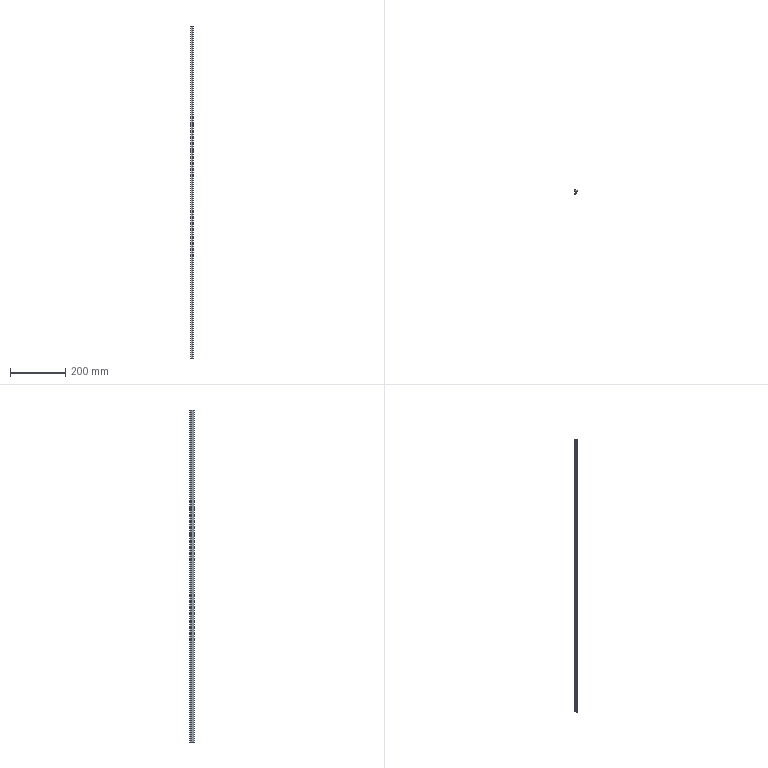Part | SolidWorks | features BaseBody 1, MoveFace 1 | 1 solid | 20 faces | box 10.8 x 17.5 x 1197 mm | volume 94324 mm3 | cylinder 11 | plane 9 | commonest cylinder face diameters 1.6 x2 14 x2 0.4 x1 0.6 x1 0.8 x1 2.6 x1
STEP:
#1=CARTESIAN_POINT('',(-3.236,-11.055,1097.));
#2=VERTEX_POINT('',#1);
#3=CARTESIAN_POINT('',(-4.3,-10.3,1097.));
#4=VERTEX_POINT('',#3);
#5=CARTESIAN_POINT('',(-3.5,-10.3,1097.));
#6=DIRECTION('',(0.,0.,-1.));
#7=DIRECTION('',(1.,0.,0.));
#8=AXIS2_PLACEMENT_3D('',#5,#6,#7);
#9=CIRCLE('',#8,0.8);
#10=EDGE_CURVE('',#2,#4,#9,.T.);
#11=ORIENTED_EDGE('',*,*,#10,.T.);
#12=CARTESIAN_POINT('',(-4.3,-10.3,-100.));
#13=VERTEX_POINT('',#12);
#14=CARTESIAN_POINT('',(-4.3,-10.3,-100.));
#15=DIRECTION('',(0.,0.,-1.));
#16=VECTOR('',#15,1000.);
#17=LINE('',#14,#16);
#18=EDGE_CURVE('',#4,#13,#17,.T.);
#19=ORIENTED_EDGE('',*,*,#18,.T.);
#20=CARTESIAN_POINT('',(-3.236,-11.055,-100.));
#21=VERTEX_POINT('',#20);
#22=CARTESIAN_POINT('',(-3.5,-10.3,-100.));
#23=DIRECTION('',(0.,0.,1.));
#24=DIRECTION('',(-1.,0.,0.));
#25=AXIS2_PLACEMENT_3D('',#22,#23,#24);
#26=CIRCLE('',#25,0.8);
#27=EDGE_CURVE('',#13,#21,#26,.T.);
#28=ORIENTED_EDGE('',*,*,#27,.T.);
#29=CARTESIAN_POINT('',(-3.236,-11.055,-100.));
#30=DIRECTION('',(0.,0.,-1.));
#31=VECTOR('',#30,1000.);
#32=LINE('',#29,#31);
#33=EDGE_CURVE('',#2,#21,#32,.T.);
#34=ORIENTED_EDGE('',*,*,#33,.F.);
#35=EDGE_LOOP('',(#11,#19,#28,#34));
#36=FACE_OUTER_BOUND('',#35,.T.);
#37=CARTESIAN_POINT('',(-3.5,-10.3,-100.));
#38=DIRECTION('',(0.,0.,-1.));
#39=DIRECTION('',(-1.,0.,0.));
#40=AXIS2_PLACEMENT_3D('',#37,#38,#39);
#41=CYLINDRICAL_SURFACE('',#40,0.8);
#42=ADVANCED_FACE('',(#36),#41,.T.);
#43=CARTESIAN_POINT('',(1.184,-6.397,-100.));
#44=VERTEX_POINT('',#43);
#45=CARTESIAN_POINT('',(-5.702,-4.29,-100.));
#46=DIRECTION('',(0.,0.,1.));
#47=DIRECTION('',(-1.,0.,0.));
#48=AXIS2_PLACEMENT_3D('',#45,#46,#47);
#49=CIRCLE('',#48,7.201);
#50=EDGE_CURVE('',#21,#44,#49,.T.);
#51=ORIENTED_EDGE('',*,*,#50,.T.);
#52=CARTESIAN_POINT('',(1.184,-6.397,1097.));
#53=VERTEX_POINT('',#52);
#54=CARTESIAN_POINT('',(1.184,-6.397,-100.));
#55=DIRECTION('',(0.,0.,1.));
#56=VECTOR('',#55,1000.);
#57=LINE('',#54,#56);
#58=EDGE_CURVE('',#44,#53,#57,.T.);
#59=ORIENTED_EDGE('',*,*,#58,.T.);
#60=CARTESIAN_POINT('',(-5.702,-4.29,1097.));
#61=DIRECTION('',(0.,0.,-1.));
#62=DIRECTION('',(1.,0.,0.));
#63=AXIS2_PLACEMENT_3D('',#60,#61,#62);
#64=CIRCLE('',#63,7.201);
#65=EDGE_CURVE('',#53,#2,#64,.T.);
#66=ORIENTED_EDGE('',*,*,#65,.T.);
#67=ORIENTED_EDGE('',*,*,#33,.T.);
#68=EDGE_LOOP('',(#51,#59,#66,#67));
#69=FACE_OUTER_BOUND('',#68,.T.);
#70=CARTESIAN_POINT('',(-5.702,-4.29,-100.));
#71=DIRECTION('',(0.,0.,-1.));
#72=DIRECTION('',(-1.,0.,0.));
#73=AXIS2_PLACEMENT_3D('',#70,#71,#72);
#74=CYLINDRICAL_SURFACE('',#73,7.201);
#75=ADVANCED_FACE('',(#69),#74,.T.);
#76=CARTESIAN_POINT('',(0.9,-6.,-100.));
#77=VERTEX_POINT('',#76);
#78=CARTESIAN_POINT('',(0.9,-6.3,-100.));
#79=DIRECTION('',(0.,0.,1.));
#80=DIRECTION('',(-1.,0.,0.));
#81=AXIS2_PLACEMENT_3D('',#78,#79,#80);
#82=CIRCLE('',#81,0.3);
#83=EDGE_CURVE('',#44,#77,#82,.T.);
#84=ORIENTED_EDGE('',*,*,#83,.T.);
#85=CARTESIAN_POINT('',(0.9,-6.,1097.));
#86=VERTEX_POINT('',#85);
#87=CARTESIAN_POINT('',(0.9,-6.,-100.));
#88=DIRECTION('',(0.,0.,1.));
#89=VECTOR('',#88,1000.);
#90=LINE('',#87,#89);
#91=EDGE_CURVE('',#77,#86,#90,.T.);
#92=ORIENTED_EDGE('',*,*,#91,.T.);
#93=CARTESIAN_POINT('',(0.9,-6.3,1097.));
#94=DIRECTION('',(0.,0.,-1.));
#95=DIRECTION('',(1.,0.,0.));
#96=AXIS2_PLACEMENT_3D('',#93,#94,#95);
#97=CIRCLE('',#96,0.3);
#98=EDGE_CURVE('',#86,#53,#97,.T.);
#99=ORIENTED_EDGE('',*,*,#98,.T.);
#100=ORIENTED_EDGE('',*,*,#58,.F.);
#101=EDGE_LOOP('',(#84,#92,#99,#100));
#102=FACE_OUTER_BOUND('',#101,.T.);
#103=CARTESIAN_POINT('',(0.9,-6.3,-100.));
#104=DIRECTION('',(0.,0.,-1.));
#105=DIRECTION('',(-1.,0.,0.));
#106=AXIS2_PLACEMENT_3D('',#103,#104,#105);
#107=CYLINDRICAL_SURFACE('',#106,0.3);
#108=ADVANCED_FACE('',(#102),#107,.T.);
#109=CARTESIAN_POINT('',(-2.5,-0.5,-100.));
#110=VERTEX_POINT('',#109);
#111=CARTESIAN_POINT('',(-2.5,-6.153,-100.));
#112=VERTEX_POINT('',#111);
#113=CARTESIAN_POINT('',(-2.5,-6.397,-100.));
#114=DIRECTION('',(0.,-1.,0.));
#115=VECTOR('',#114,1000.);
#116=LINE('',#113,#115);
#117=EDGE_CURVE('',#110,#112,#116,.T.);
#118=ORIENTED_EDGE('',*,*,#117,.F.);
#119=CARTESIAN_POINT('',(-4.2,1.695,-100.));
#120=VERTEX_POINT('',#119);
#121=CARTESIAN_POINT('',(-1.701,1.875,-100.));
#122=DIRECTION('',(0.,0.,1.));
#123=DIRECTION('',(-1.,0.,0.));
#124=AXIS2_PLACEMENT_3D('',#121,#122,#123);
#125=CIRCLE('',#124,2.506);
#126=EDGE_CURVE('',#120,#110,#125,.T.);
#127=ORIENTED_EDGE('',*,*,#126,.F.);
#128=CARTESIAN_POINT('',(-4.2,5.1,-100.));
#129=VERTEX_POINT('',#128);
#130=CARTESIAN_POINT('',(-4.2,-6.397,-100.));
#131=DIRECTION('',(0.,-1.,0.));
#132=VECTOR('',#131,1000.);
#133=LINE('',#130,#132);
#134=EDGE_CURVE('',#129,#120,#133,.T.);
#135=ORIENTED_EDGE('',*,*,#134,.F.);
#136=CARTESIAN_POINT('',(-2.892,6.4,-100.));
#137=VERTEX_POINT('',#136);
#138=CARTESIAN_POINT('',(-2.9,5.1,-100.));
#139=DIRECTION('',(0.,0.,1.));
#140=DIRECTION('',(-1.,0.,0.));
#141=AXIS2_PLACEMENT_3D('',#138,#139,#140);
#142=CIRCLE('',#141,1.3);
#143=EDGE_CURVE('',#137,#129,#142,.T.);
#144=ORIENTED_EDGE('',*,*,#143,.F.);
#145=CARTESIAN_POINT('',(0.5,5.5,-100.));
#146=VERTEX_POINT('',#145);
#147=CARTESIAN_POINT('',(-2.934,-0.5999,-100.));
#148=DIRECTION('',(0.,0.,1.));
#149=DIRECTION('',(-1.,0.,0.));
#150=AXIS2_PLACEMENT_3D('',#147,#148,#149);
#151=CIRCLE('',#150,7.);
#152=EDGE_CURVE('',#146,#137,#151,.T.);
#153=ORIENTED_EDGE('',*,*,#152,.F.);
#154=CARTESIAN_POINT('',(5.5,1.7,-100.));
#155=VERTEX_POINT('',#154);
#156=CARTESIAN_POINT('',(5.5,1.7,-100.));
#157=DIRECTION('',(-0.7962,0.6051,0.));
#158=VECTOR('',#157,1000.);
#159=LINE('',#156,#158);
#160=EDGE_CURVE('',#155,#146,#159,.T.);
#161=ORIENTED_EDGE('',*,*,#160,.F.);
#162=CARTESIAN_POINT('',(6.458,-0.2215,-100.));
#163=VERTEX_POINT('',#162);
#164=CARTESIAN_POINT('',(6.458,-0.2215,-100.));
#165=DIRECTION('',(-0.4462,0.8949,0.));
#166=VECTOR('',#165,1000.);
#167=LINE('',#164,#166);
#168=EDGE_CURVE('',#163,#155,#167,.T.);
#169=ORIENTED_EDGE('',*,*,#168,.F.);
#170=CARTESIAN_POINT('',(5.895,-0.7433,-100.));
#171=VERTEX_POINT('',#170);
#172=CARTESIAN_POINT('',(6.1,-0.4,-100.));
#173=DIRECTION('',(0.,0.,1.));
#174=DIRECTION('',(-1.,0.,0.));
#175=AXIS2_PLACEMENT_3D('',#172,#173,#174);
#176=CIRCLE('',#175,0.4);
#177=EDGE_CURVE('',#171,#163,#176,.T.);
#178=ORIENTED_EDGE('',*,*,#177,.F.);
#179=CARTESIAN_POINT('',(3.,0.,-100.));
#180=VERTEX_POINT('',#179);
#181=CARTESIAN_POINT('',(2.746,-6.995,-100.));
#182=DIRECTION('',(0.,0.,-1.));
#183=DIRECTION('',(-1.,0.,0.));
#184=AXIS2_PLACEMENT_3D('',#181,#182,#183);
#185=CIRCLE('',#184,7.);
#186=EDGE_CURVE('',#180,#171,#185,.T.);
#187=ORIENTED_EDGE('',*,*,#186,.F.);
#188=CARTESIAN_POINT('',(0.,0.,-100.));
#189=VERTEX_POINT('',#188);
#190=CARTESIAN_POINT('',(-6.814,0.,-100.));
#191=DIRECTION('',(1.,0.,0.));
#192=VECTOR('',#191,1000.);
#193=LINE('',#190,#192);
#194=EDGE_CURVE('',#189,#180,#193,.T.);
#195=ORIENTED_EDGE('',*,*,#194,.F.);
#196=CARTESIAN_POINT('',(0.,-5.8,-100.));
#197=VERTEX_POINT('',#196);
#198=CARTESIAN_POINT('',(0.,-6.397,-100.));
#199=DIRECTION('',(0.,1.,0.));
#200=VECTOR('',#199,1000.);
#201=LINE('',#198,#200);
#202=EDGE_CURVE('',#197,#189,#201,.T.);
#203=ORIENTED_EDGE('',*,*,#202,.F.);
#204=CARTESIAN_POINT('',(0.2,-6.,-100.));
#205=VERTEX_POINT('',#204);
#206=CARTESIAN_POINT('',(0.2,-5.8,-100.));
#207=DIRECTION('',(0.,0.,1.));
#208=DIRECTION('',(-1.,0.,0.));
#209=AXIS2_PLACEMENT_3D('',#206,#207,#208);
#210=CIRCLE('',#209,0.2);
#211=EDGE_CURVE('',#197,#205,#210,.T.);
#212=ORIENTED_EDGE('',*,*,#211,.T.);
#213=CARTESIAN_POINT('',(-6.814,-6.,-100.));
#214=DIRECTION('',(-1.,0.,0.));
#215=VECTOR('',#214,1000.);
#216=LINE('',#213,#215);
#217=EDGE_CURVE('',#77,#205,#216,.T.);
#218=ORIENTED_EDGE('',*,*,#217,.F.);
#219=ORIENTED_EDGE('',*,*,#83,.F.);
#220=ORIENTED_EDGE('',*,*,#50,.F.);
#221=ORIENTED_EDGE('',*,*,#27,.F.);
#222=CARTESIAN_POINT('',(-3.998,-9.674,-100.));
#223=VERTEX_POINT('',#222);
#224=CARTESIAN_POINT('',(-3.5,-10.3,-100.));
#225=DIRECTION('',(0.,0.,1.));
#226=DIRECTION('',(-1.,0.,0.));
#227=AXIS2_PLACEMENT_3D('',#224,#225,#226);
#228=CIRCLE('',#227,0.8);
#229=EDGE_CURVE('',#223,#13,#228,.T.);
#230=ORIENTED_EDGE('',*,*,#229,.F.);
#231=CARTESIAN_POINT('',(-6.814,-6.397,-100.));
#232=DIRECTION('',(0.,0.,-1.));
#233=DIRECTION('',(-1.,0.,0.));
#234=AXIS2_PLACEMENT_3D('',#231,#232,#233);
#235=CIRCLE('',#234,4.321);
#236=EDGE_CURVE('',#112,#223,#235,.T.);
#237=ORIENTED_EDGE('',*,*,#236,.F.);
#238=EDGE_LOOP('',(#118,#127,#135,#144,#153,#161,#169,#178,#187,#195,#203,#212,#218,#219,#220,#221,#230,#237));
#239=FACE_OUTER_BOUND('',#238,.T.);
#240=CARTESIAN_POINT('',(-6.814,-6.397,-100.));
#241=DIRECTION('',(0.,0.,1.));
#242=DIRECTION('',(1.,0.,0.));
#243=AXIS2_PLACEMENT_3D('',#240,#241,#242);
#244=PLANE('',#243);
#245=ADVANCED_FACE('',(#239),#244,.F.);
#246=ORIENTED_EDGE('',*,*,#18,.F.);
#247=CARTESIAN_POINT('',(-3.998,-9.674,1097.));
#248=VERTEX_POINT('',#247);
#249=CARTESIAN_POINT('',(-3.5,-10.3,1097.));
#250=DIRECTION('',(0.,0.,-1.));
#251=DIRECTION('',(1.,0.,0.));
#252=AXIS2_PLACEMENT_3D('',#249,#250,#251);
#253=CIRCLE('',#252,0.8);
#254=EDGE_CURVE('',#4,#248,#253,.T.);
#255=ORIENTED_EDGE('',*,*,#254,.T.);
#256=CARTESIAN_POINT('',(-3.998,-9.674,-100.));
#257=DIRECTION('',(0.,0.,-1.));
#258=VECTOR('',#257,1000.);
#259=LINE('',#256,#258);
#260=EDGE_CURVE('',#248,#223,#259,.T.);
#261=ORIENTED_EDGE('',*,*,#260,.T.);
#262=ORIENTED_EDGE('',*,*,#229,.T.);
#263=EDGE_LOOP('',(#246,#255,#261,#262));
#264=FACE_OUTER_BOUND('',#263,.T.);
#265=CARTESIAN_POINT('',(-3.5,-10.3,-100.));
#266=DIRECTION('',(0.,0.,-1.));
#267=DIRECTION('',(-1.,0.,0.));
#268=AXIS2_PLACEMENT_3D('',#265,#266,#267);
#269=CYLINDRICAL_SURFACE('',#268,0.8);
#270=ADVANCED_FACE('',(#264),#269,.T.);
#271=CARTESIAN_POINT('',(-4.2,1.695,1097.));
#272=VERTEX_POINT('',#271);
#273=CARTESIAN_POINT('',(-2.5,-0.5,1097.));
#274=VERTEX_POINT('',#273);
#275=CARTESIAN_POINT('',(-1.701,1.875,1097.));
#276=DIRECTION('',(0.,0.,1.));
#277=DIRECTION('',(1.,0.,0.));
#278=AXIS2_PLACEMENT_3D('',#275,#276,#277);
#279=CIRCLE('',#278,2.506);
#280=EDGE_CURVE('',#272,#274,#279,.T.);
#281=ORIENTED_EDGE('',*,*,#280,.T.);
#282=CARTESIAN_POINT('',(-2.5,-6.153,1097.));
#283=VERTEX_POINT('',#282);
#284=CARTESIAN_POINT('',(-2.5,-6.397,1097.));
#285=DIRECTION('',(0.,-1.,0.));
#286=VECTOR('',#285,1000.);
#287=LINE('',#284,#286);
#288=EDGE_CURVE('',#274,#283,#287,.T.);
#289=ORIENTED_EDGE('',*,*,#288,.T.);
#290=CARTESIAN_POINT('',(-6.814,-6.397,1097.));
#291=DIRECTION('',(0.,0.,-1.));
#292=DIRECTION('',(1.,0.,0.));
#293=AXIS2_PLACEMENT_3D('',#290,#291,#292);
#294=CIRCLE('',#293,4.321);
#295=EDGE_CURVE('',#283,#248,#294,.T.);
#296=ORIENTED_EDGE('',*,*,#295,.T.);
#297=ORIENTED_EDGE('',*,*,#254,.F.);
#298=ORIENTED_EDGE('',*,*,#10,.F.);
#299=ORIENTED_EDGE('',*,*,#65,.F.);
#300=ORIENTED_EDGE('',*,*,#98,.F.);
#301=CARTESIAN_POINT('',(0.2,-6.,1097.));
#302=VERTEX_POINT('',#301);
#303=CARTESIAN_POINT('',(-6.814,-6.,1097.));
#304=DIRECTION('',(-1.,0.,0.));
#305=VECTOR('',#304,1000.);
#306=LINE('',#303,#305);
#307=EDGE_CURVE('',#86,#302,#306,.T.);
#308=ORIENTED_EDGE('',*,*,#307,.T.);
#309=CARTESIAN_POINT('',(0.,-5.8,1097.));
#310=VERTEX_POINT('',#309);
#311=CARTESIAN_POINT('',(0.2,-5.8,1097.));
#312=DIRECTION('',(0.,0.,-1.));
#313=DIRECTION('',(1.,0.,0.));
#314=AXIS2_PLACEMENT_3D('',#311,#312,#313);
#315=CIRCLE('',#314,0.2);
#316=EDGE_CURVE('',#302,#310,#315,.T.);
#317=ORIENTED_EDGE('',*,*,#316,.T.);
#318=CARTESIAN_POINT('',(0.,0.,1097.));
#319=VERTEX_POINT('',#318);
#320=CARTESIAN_POINT('',(0.,-6.397,1097.));
#321=DIRECTION('',(0.,1.,0.));
#322=VECTOR('',#321,1000.);
#323=LINE('',#320,#322);
#324=EDGE_CURVE('',#310,#319,#323,.T.);
#325=ORIENTED_EDGE('',*,*,#324,.T.);
#326=CARTESIAN_POINT('',(3.,0.,1097.));
#327=VERTEX_POINT('',#326);
#328=CARTESIAN_POINT('',(-6.814,0.,1097.));
#329=DIRECTION('',(1.,0.,0.));
#330=VECTOR('',#329,1000.);
#331=LINE('',#328,#330);
#332=EDGE_CURVE('',#319,#327,#331,.T.);
#333=ORIENTED_EDGE('',*,*,#332,.T.);
#334=CARTESIAN_POINT('',(5.895,-0.7433,1097.));
#335=VERTEX_POINT('',#334);
#336=CARTESIAN_POINT('',(2.746,-6.995,1097.));
#337=DIRECTION('',(0.,0.,-1.));
#338=DIRECTION('',(1.,0.,0.));
#339=AXIS2_PLACEMENT_3D('',#336,#337,#338);
#340=CIRCLE('',#339,7.);
#341=EDGE_CURVE('',#327,#335,#340,.T.);
#342=ORIENTED_EDGE('',*,*,#341,.T.);
#343=CARTESIAN_POINT('',(6.458,-0.2215,1097.));
#344=VERTEX_POINT('',#343);
#345=CARTESIAN_POINT('',(6.1,-0.4,1097.));
#346=DIRECTION('',(0.,0.,-1.));
#347=DIRECTION('',(1.,0.,0.));
#348=AXIS2_PLACEMENT_3D('',#345,#346,#347);
#349=CIRCLE('',#348,0.4);
#350=EDGE_CURVE('',#344,#335,#349,.T.);
#351=ORIENTED_EDGE('',*,*,#350,.F.);
#352=CARTESIAN_POINT('',(5.5,1.7,1097.));
#353=VERTEX_POINT('',#352);
#354=CARTESIAN_POINT('',(6.282,0.1323,1097.));
#355=DIRECTION('',(-0.4462,0.8949,0.));
#356=VECTOR('',#355,1000.);
#357=LINE('',#354,#356);
#358=EDGE_CURVE('',#344,#353,#357,.T.);
#359=ORIENTED_EDGE('',*,*,#358,.T.);
#360=CARTESIAN_POINT('',(0.5,5.5,1097.));
#361=VERTEX_POINT('',#360);
#362=CARTESIAN_POINT('',(1.595,4.668,1097.));
#363=DIRECTION('',(-0.7962,0.6051,0.));
#364=VECTOR('',#363,1000.);
#365=LINE('',#362,#364);
#366=EDGE_CURVE('',#353,#361,#365,.T.);
#367=ORIENTED_EDGE('',*,*,#366,.T.);
#368=CARTESIAN_POINT('',(-2.892,6.4,1097.));
#369=VERTEX_POINT('',#368);
#370=CARTESIAN_POINT('',(-2.934,-0.5999,1097.));
#371=DIRECTION('',(0.,0.,1.));
#372=DIRECTION('',(1.,0.,0.));
#373=AXIS2_PLACEMENT_3D('',#370,#371,#372);
#374=CIRCLE('',#373,7.);
#375=EDGE_CURVE('',#361,#369,#374,.T.);
#376=ORIENTED_EDGE('',*,*,#375,.T.);
#377=CARTESIAN_POINT('',(-4.2,5.1,1097.));
#378=VERTEX_POINT('',#377);
#379=CARTESIAN_POINT('',(-2.9,5.1,1097.));
#380=DIRECTION('',(0.,0.,1.));
#381=DIRECTION('',(1.,0.,0.));
#382=AXIS2_PLACEMENT_3D('',#379,#380,#381);
#383=CIRCLE('',#382,1.3);
#384=EDGE_CURVE('',#369,#378,#383,.T.);
#385=ORIENTED_EDGE('',*,*,#384,.T.);
#386=CARTESIAN_POINT('',(-4.2,-6.397,1097.));
#387=DIRECTION('',(0.,-1.,0.));
#388=VECTOR('',#387,1000.);
#389=LINE('',#386,#388);
#390=EDGE_CURVE('',#378,#272,#389,.T.);
#391=ORIENTED_EDGE('',*,*,#390,.T.);
#392=EDGE_LOOP('',(#281,#289,#296,#297,#298,#299,#300,#308,#317,#325,#333,#342,#351,#359,#367,#376,#385,#391));
#393=FACE_OUTER_BOUND('',#392,.T.);
#394=CARTESIAN_POINT('',(-6.814,-6.397,1097.));
#395=DIRECTION('',(0.,0.,1.));
#396=DIRECTION('',(1.,0.,0.));
#397=AXIS2_PLACEMENT_3D('',#394,#395,#396);
#398=PLANE('',#397);
#399=ADVANCED_FACE('',(#393),#398,.T.);
#400=ORIENTED_EDGE('',*,*,#217,.T.);
#401=CARTESIAN_POINT('',(0.2,-6.,-100.));
#402=DIRECTION('',(0.,0.,1.));
#403=VECTOR('',#402,1000.);
#404=LINE('',#401,#403);
#405=EDGE_CURVE('',#205,#302,#404,.T.);
#406=ORIENTED_EDGE('',*,*,#405,.T.);
#407=ORIENTED_EDGE('',*,*,#307,.F.);
#408=ORIENTED_EDGE('',*,*,#91,.F.);
#409=EDGE_LOOP('',(#400,#406,#407,#408));
#410=FACE_OUTER_BOUND('',#409,.T.);
#411=CARTESIAN_POINT('',(0.9,-6.,-100.));
#412=DIRECTION('',(0.,1.,0.));
#413=DIRECTION('',(0.,0.,1.));
#414=AXIS2_PLACEMENT_3D('',#411,#412,#413);
#415=PLANE('',#414);
#416=ADVANCED_FACE('',(#410),#415,.T.);
#417=CARTESIAN_POINT('',(-2.5,-6.153,-100.));
#418=DIRECTION('',(0.,0.,1.));
#419=VECTOR('',#418,1000.);
#420=LINE('',#417,#419);
#421=EDGE_CURVE('',#112,#283,#420,.T.);
#422=ORIENTED_EDGE('',*,*,#421,.F.);
#423=ORIENTED_EDGE('',*,*,#236,.T.);
#424=ORIENTED_EDGE('',*,*,#260,.F.);
#425=ORIENTED_EDGE('',*,*,#295,.F.);
#426=EDGE_LOOP('',(#422,#423,#424,#425));
#427=FACE_OUTER_BOUND('',#426,.T.);
#428=CARTESIAN_POINT('',(-6.814,-6.397,-100.));
#429=DIRECTION('',(0.,0.,-1.));
#430=DIRECTION('',(-1.,0.,0.));
#431=AXIS2_PLACEMENT_3D('',#428,#429,#430);
#432=CYLINDRICAL_SURFACE('',#431,4.321);
#433=ADVANCED_FACE('',(#427),#432,.F.);
#434=ORIENTED_EDGE('',*,*,#117,.T.);
#435=ORIENTED_EDGE('',*,*,#421,.T.);
#436=ORIENTED_EDGE('',*,*,#288,.F.);
#437=CARTESIAN_POINT('',(-2.5,-0.5,-100.));
#438=DIRECTION('',(0.,0.,-1.));
#439=VECTOR('',#438,1000.);
#440=LINE('',#437,#439);
#441=EDGE_CURVE('',#274,#110,#440,.T.);
#442=ORIENTED_EDGE('',*,*,#441,.T.);
#443=EDGE_LOOP('',(#434,#435,#436,#442));
#444=FACE_OUTER_BOUND('',#443,.T.);
#445=CARTESIAN_POINT('',(-2.5,-0.5,-100.));
#446=DIRECTION('',(-1.,0.,0.));
#447=DIRECTION('',(0.,0.,1.));
#448=AXIS2_PLACEMENT_3D('',#445,#446,#447);
#449=PLANE('',#448);
#450=ADVANCED_FACE('',(#444),#449,.T.);
#451=ORIENTED_EDGE('',*,*,#126,.T.);
#452=ORIENTED_EDGE('',*,*,#441,.F.);
#453=ORIENTED_EDGE('',*,*,#280,.F.);
#454=CARTESIAN_POINT('',(-4.2,1.695,-100.));
#455=DIRECTION('',(0.,0.,-1.));
#456=VECTOR('',#455,1000.);
#457=LINE('',#454,#456);
#458=EDGE_CURVE('',#272,#120,#457,.T.);
#459=ORIENTED_EDGE('',*,*,#458,.T.);
#460=EDGE_LOOP('',(#451,#452,#453,#459));
#461=FACE_OUTER_BOUND('',#460,.T.);
#462=CARTESIAN_POINT('',(-1.701,1.875,-100.));
#463=DIRECTION('',(0.,0.,-1.));
#464=DIRECTION('',(-1.,0.,0.));
#465=AXIS2_PLACEMENT_3D('',#462,#463,#464);
#466=CYLINDRICAL_SURFACE('',#465,2.506);
#467=ADVANCED_FACE('',(#461),#466,.T.);
#468=ORIENTED_EDGE('',*,*,#134,.T.);
#469=ORIENTED_EDGE('',*,*,#458,.F.);
#470=ORIENTED_EDGE('',*,*,#390,.F.);
#471=CARTESIAN_POINT('',(-4.2,5.1,-100.));
#472=DIRECTION('',(0.,0.,-1.));
#473=VECTOR('',#472,1000.);
#474=LINE('',#471,#473);
#475=EDGE_CURVE('',#378,#129,#474,.T.);
#476=ORIENTED_EDGE('',*,*,#475,.T.);
#477=EDGE_LOOP('',(#468,#469,#470,#476));
#478=FACE_OUTER_BOUND('',#477,.T.);
#479=CARTESIAN_POINT('',(-4.2,5.1,-100.));
#480=DIRECTION('',(-1.,0.,0.));
#481=DIRECTION('',(0.,0.,1.));
#482=AXIS2_PLACEMENT_3D('',#479,#480,#481);
#483=PLANE('',#482);
#484=ADVANCED_FACE('',(#478),#483,.T.);
#485=ORIENTED_EDGE('',*,*,#143,.T.);
#486=ORIENTED_EDGE('',*,*,#475,.F.);
#487=ORIENTED_EDGE('',*,*,#384,.F.);
#488=CARTESIAN_POINT('',(-2.892,6.4,-100.));
#489=DIRECTION('',(0.,0.,-1.));
#490=VECTOR('',#489,1000.);
#491=LINE('',#488,#490);
#492=EDGE_CURVE('',#369,#137,#491,.T.);
#493=ORIENTED_EDGE('',*,*,#492,.T.);
#494=EDGE_LOOP('',(#485,#486,#487,#493));
#495=FACE_OUTER_BOUND('',#494,.T.);
#496=CARTESIAN_POINT('',(-2.9,5.1,-100.));
#497=DIRECTION('',(0.,0.,-1.));
#498=DIRECTION('',(-1.,0.,0.));
#499=AXIS2_PLACEMENT_3D('',#496,#497,#498);
#500=CYLINDRICAL_SURFACE('',#499,1.3);
#501=ADVANCED_FACE('',(#495),#500,.T.);
#502=ORIENTED_EDGE('',*,*,#152,.T.);
#503=ORIENTED_EDGE('',*,*,#492,.F.);
#504=ORIENTED_EDGE('',*,*,#375,.F.);
#505=CARTESIAN_POINT('',(0.5,5.5,-100.));
#506=DIRECTION('',(0.,0.,-1.));
#507=VECTOR('',#506,1000.);
#508=LINE('',#505,#507);
#509=EDGE_CURVE('',#361,#146,#508,.T.);
#510=ORIENTED_EDGE('',*,*,#509,.T.);
#511=EDGE_LOOP('',(#502,#503,#504,#510));
#512=FACE_OUTER_BOUND('',#511,.T.);
#513=CARTESIAN_POINT('',(-2.934,-0.5999,-100.));
#514=DIRECTION('',(0.,0.,-1.));
#515=DIRECTION('',(-1.,0.,0.));
#516=AXIS2_PLACEMENT_3D('',#513,#514,#515);
#517=CYLINDRICAL_SURFACE('',#516,7.);
#518=ADVANCED_FACE('',(#512),#517,.T.);
#519=ORIENTED_EDGE('',*,*,#160,.T.);
#520=ORIENTED_EDGE('',*,*,#509,.F.);
#521=ORIENTED_EDGE('',*,*,#366,.F.);
#522=CARTESIAN_POINT('',(5.5,1.7,-100.));
#523=DIRECTION('',(0.,0.,-1.));
#524=VECTOR('',#523,1000.);
#525=LINE('',#522,#524);
#526=EDGE_CURVE('',#353,#155,#525,.T.);
#527=ORIENTED_EDGE('',*,*,#526,.T.);
#528=EDGE_LOOP('',(#519,#520,#521,#527));
#529=FACE_OUTER_BOUND('',#528,.T.);
#530=CARTESIAN_POINT('',(5.5,1.7,-100.));
#531=DIRECTION('',(0.6051,0.7962,0.));
#532=DIRECTION('',(-0.7962,0.6051,0.));
#533=AXIS2_PLACEMENT_3D('',#530,#531,#532);
#534=PLANE('',#533);
#535=ADVANCED_FACE('',(#529),#534,.T.);
#536=ORIENTED_EDGE('',*,*,#168,.T.);
#537=ORIENTED_EDGE('',*,*,#526,.F.);
#538=ORIENTED_EDGE('',*,*,#358,.F.);
#539=CARTESIAN_POINT('',(6.458,-0.2215,-100.));
#540=DIRECTION('',(0.,0.,-1.));
#541=VECTOR('',#540,1000.);
#542=LINE('',#539,#541);
#543=EDGE_CURVE('',#344,#163,#542,.T.);
#544=ORIENTED_EDGE('',*,*,#543,.T.);
#545=EDGE_LOOP('',(#536,#537,#538,#544));
#546=FACE_OUTER_BOUND('',#545,.T.);
#547=CARTESIAN_POINT('',(6.458,-0.2215,-100.));
#548=DIRECTION('',(0.8949,0.4462,0.));
#549=DIRECTION('',(-0.4462,0.8949,0.));
#550=AXIS2_PLACEMENT_3D('',#547,#548,#549);
#551=PLANE('',#550);
#552=ADVANCED_FACE('',(#546),#551,.T.);
#553=CARTESIAN_POINT('',(3.,0.,-100.));
#554=DIRECTION('',(0.,0.,1.));
#555=VECTOR('',#554,1000.);
#556=LINE('',#553,#555);
#557=EDGE_CURVE('',#180,#327,#556,.T.);
#558=ORIENTED_EDGE('',*,*,#557,.F.);
#559=ORIENTED_EDGE('',*,*,#186,.T.);
#560=CARTESIAN_POINT('',(5.895,-0.7433,-100.));
#561=DIRECTION('',(0.,0.,-1.));
#562=VECTOR('',#561,1000.);
#563=LINE('',#560,#562);
#564=EDGE_CURVE('',#335,#171,#563,.T.);
#565=ORIENTED_EDGE('',*,*,#564,.F.);
#566=ORIENTED_EDGE('',*,*,#341,.F.);
#567=EDGE_LOOP('',(#558,#559,#565,#566));
#568=FACE_OUTER_BOUND('',#567,.T.);
#569=CARTESIAN_POINT('',(2.746,-6.995,-100.));
#570=DIRECTION('',(0.,0.,-1.));
#571=DIRECTION('',(-1.,0.,0.));
#572=AXIS2_PLACEMENT_3D('',#569,#570,#571);
#573=CYLINDRICAL_SURFACE('',#572,7.);
#574=ADVANCED_FACE('',(#568),#573,.F.);
#575=ORIENTED_EDGE('',*,*,#194,.T.);
#576=ORIENTED_EDGE('',*,*,#557,.T.);
#577=ORIENTED_EDGE('',*,*,#332,.F.);
#578=CARTESIAN_POINT('',(0.,0.,-100.));
#579=DIRECTION('',(0.,0.,-1.));
#580=VECTOR('',#579,1000.);
#581=LINE('',#578,#580);
#582=EDGE_CURVE('',#319,#189,#581,.T.);
#583=ORIENTED_EDGE('',*,*,#582,.T.);
#584=EDGE_LOOP('',(#575,#576,#577,#583));
#585=FACE_OUTER_BOUND('',#584,.T.);
#586=CARTESIAN_POINT('',(0.,0.,-100.));
#587=DIRECTION('',(0.,-1.,0.));
#588=DIRECTION('',(0.,0.,-1.));
#589=AXIS2_PLACEMENT_3D('',#586,#587,#588);
#590=PLANE('',#589);
#591=ADVANCED_FACE('',(#585),#590,.T.);
#592=ORIENTED_EDGE('',*,*,#202,.T.);
#593=ORIENTED_EDGE('',*,*,#582,.F.);
#594=ORIENTED_EDGE('',*,*,#324,.F.);
#595=CARTESIAN_POINT('',(0.,-5.8,-100.));
#596=DIRECTION('',(0.,0.,-1.));
#597=VECTOR('',#596,1000.);
#598=LINE('',#595,#597);
#599=EDGE_CURVE('',#310,#197,#598,.T.);
#600=ORIENTED_EDGE('',*,*,#599,.T.);
#601=EDGE_LOOP('',(#592,#593,#594,#600));
#602=FACE_OUTER_BOUND('',#601,.T.);
#603=CARTESIAN_POINT('',(0.,-5.8,-100.));
#604=DIRECTION('',(1.,0.,0.));
#605=DIRECTION('',(0.,0.,-1.));
#606=AXIS2_PLACEMENT_3D('',#603,#604,#605);
#607=PLANE('',#606);
#608=ADVANCED_FACE('',(#602),#607,.T.);
#609=ORIENTED_EDGE('',*,*,#405,.F.);
#610=ORIENTED_EDGE('',*,*,#211,.F.);
#611=ORIENTED_EDGE('',*,*,#599,.F.);
#612=ORIENTED_EDGE('',*,*,#316,.F.);
#613=EDGE_LOOP('',(#609,#610,#611,#612));
#614=FACE_OUTER_BOUND('',#613,.T.);
#615=CARTESIAN_POINT('',(0.2,-5.8,-100.));
#616=DIRECTION('',(0.,0.,-1.));
#617=DIRECTION('',(-1.,0.,0.));
#618=AXIS2_PLACEMENT_3D('',#615,#616,#617);
#619=CYLINDRICAL_SURFACE('',#618,0.2);
#620=ADVANCED_FACE('',(#614),#619,.F.);
#621=ORIENTED_EDGE('',*,*,#177,.T.);
#622=ORIENTED_EDGE('',*,*,#543,.F.);
#623=ORIENTED_EDGE('',*,*,#350,.T.);
#624=ORIENTED_EDGE('',*,*,#564,.T.);
#625=EDGE_LOOP('',(#621,#622,#623,#624));
#626=FACE_OUTER_BOUND('',#625,.T.);
#627=CARTESIAN_POINT('',(6.1,-0.4,-100.));
#628=DIRECTION('',(0.,0.,-1.));
#629=DIRECTION('',(-1.,0.,0.));
#630=AXIS2_PLACEMENT_3D('',#627,#628,#629);
#631=CYLINDRICAL_SURFACE('',#630,0.4);
#632=ADVANCED_FACE('',(#626),#631,.T.);
#633=CLOSED_SHELL('',(#42,#75,#108,#245,#270,#399,#416,#433,#450,#467,#484,#501,#518,#535,#552,#574,#591,#608,#620,#632));
#634=MANIFOLD_SOLID_BREP('',#633);
#635=CARTESIAN_POINT('',(0.,0.,0.));
#636=DIRECTION('',(0.,0.,1.));
#637=DIRECTION('',(1.,0.,0.));
#638=AXIS2_PLACEMENT_3D('',#635,#636,#637);
#639=(LENGTH_UNIT()NAMED_UNIT(*)SI_UNIT(.MILLI.,.METRE.));
#640=UNCERTAINTY_MEASURE_WITH_UNIT(LENGTH_MEASURE(0.00001),#639,'','');
#641=(NAMED_UNIT(*)PLANE_ANGLE_UNIT()SI_UNIT($,.RADIAN.));
#642=(NAMED_UNIT(*)SI_UNIT($,.STERADIAN.)SOLID_ANGLE_UNIT());
#643=(GEOMETRIC_REPRESENTATION_CONTEXT(3)GLOBAL_UNCERTAINTY_ASSIGNED_CONTEXT((#640))GLOBAL_UNIT_ASSIGNED_CONTEXT((#639,#641,#642))REPRESENTATION_CONTEXT('',''));
#644=ADVANCED_BREP_SHAPE_REPRESENTATION('',(#634,#638),#643);